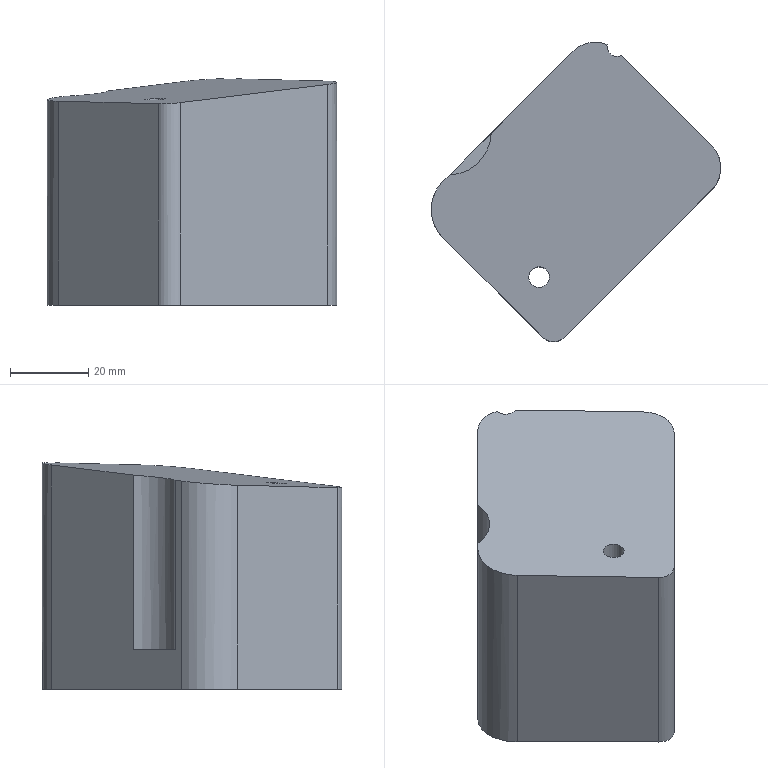Part | STEP file | gslz 2016.10.28-13_id1354_x_t | 1 solid | 14 faces | box 73.861 x 76.347 x 57.728 mm | volume 171700 mm3 | cylinder 7 | plane 6 | spline 1 | commonest cylinder face diameters 5.3 x2 16 x2 8 x1 20 x1 22 x1